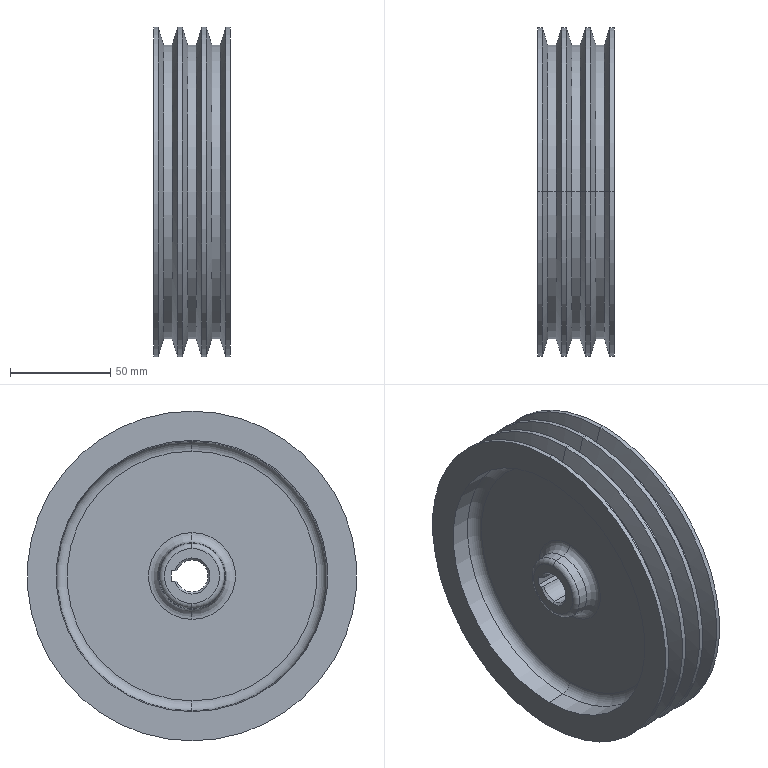Part | SolidWorks | features Fillet 2, Chamfer 1, Cut 1, LPattern 1, RevCut 1, Revolution 1 | 1 solid | 64 faces | box 38 x 164 x 164 mm | volume 318015 mm3 | cone 26 | cylinder 17 | torus 12 | plane 9 | commonest cylinder face diameters 164 x8 146 x6 16 x3